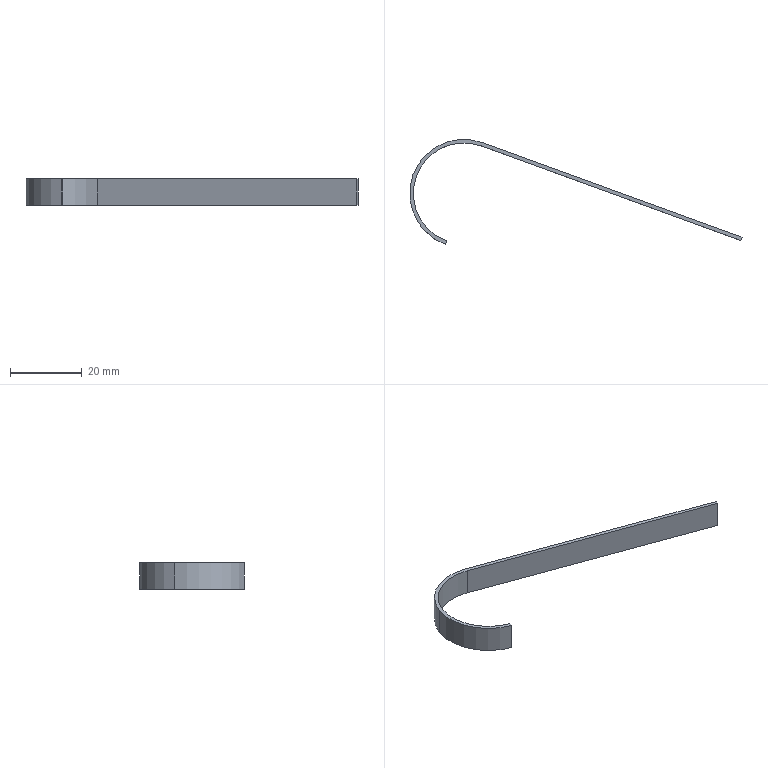Part | SolidWorks | features SplitBody 1 | 1 solid | 10 faces | box 92.373 x 29.202 x 7.5 mm | volume 918.944 mm3 | plane 6 | cylinder 4 | commonest cylinder face diameters 28.11 x2 30.11 x2
STEP:
#1=CARTESIAN_POINT('',(-138.829,345.94,-434.002));
#2=VERTEX_POINT('',#1);
#3=CARTESIAN_POINT('',(-156.843,337.54,-434.002));
#4=VERTEX_POINT('',#3);
#5=CARTESIAN_POINT('',(-143.636,332.733,-434.002));
#6=DIRECTION('',(0.,0.,1.));
#7=DIRECTION('',(0.9397,-0.342,0.));
#8=AXIS2_PLACEMENT_3D('',#5,#6,#7);
#9=CIRCLE('',#8,14.055);
#10=EDGE_CURVE('',#2,#4,#9,.T.);
#11=ORIENTED_EDGE('',*,*,#10,.T.);
#12=CARTESIAN_POINT('',(-156.843,337.54,-441.502));
#13=VERTEX_POINT('',#12);
#14=CARTESIAN_POINT('',(-156.843,337.54,-434.002));
#15=DIRECTION('',(0.,0.,-1.));
#16=VECTOR('',#15,1000.);
#17=LINE('',#14,#16);
#18=EDGE_CURVE('',#4,#13,#17,.T.);
#19=ORIENTED_EDGE('',*,*,#18,.T.);
#20=CARTESIAN_POINT('',(-138.829,345.94,-441.502));
#21=VERTEX_POINT('',#20);
#22=CARTESIAN_POINT('',(-143.636,332.733,-441.502));
#23=DIRECTION('',(0.,0.,1.));
#24=DIRECTION('',(0.9397,-0.342,0.));
#25=AXIS2_PLACEMENT_3D('',#22,#23,#24);
#26=CIRCLE('',#25,14.055);
#27=EDGE_CURVE('',#21,#13,#26,.T.);
#28=ORIENTED_EDGE('',*,*,#27,.F.);
#29=CARTESIAN_POINT('',(-138.829,345.94,-434.002));
#30=DIRECTION('',(0.,0.,-1.));
#31=VECTOR('',#30,1000.);
#32=LINE('',#29,#31);
#33=EDGE_CURVE('',#2,#21,#32,.T.);
#34=ORIENTED_EDGE('',*,*,#33,.F.);
#35=EDGE_LOOP('',(#11,#19,#28,#34));
#36=FACE_OUTER_BOUND('',#35,.T.);
#37=CARTESIAN_POINT('',(-143.636,332.733,-434.002));
#38=DIRECTION('',(0.,0.,-1.));
#39=DIRECTION('',(-0.9397,0.342,0.));
#40=AXIS2_PLACEMENT_3D('',#37,#38,#39);
#41=CYLINDRICAL_SURFACE('',#40,14.055);
#42=ADVANCED_FACE('',(#36),#41,.F.);
#43=CARTESIAN_POINT('',(-157.783,337.882,-434.002));
#44=VERTEX_POINT('',#43);
#45=CARTESIAN_POINT('',(-148.785,318.586,-434.002));
#46=VERTEX_POINT('',#45);
#47=CARTESIAN_POINT('',(-143.636,332.733,-434.002));
#48=DIRECTION('',(0.,0.,1.));
#49=DIRECTION('',(0.9397,-0.342,0.));
#50=AXIS2_PLACEMENT_3D('',#47,#48,#49);
#51=CIRCLE('',#50,15.055);
#52=EDGE_CURVE('',#44,#46,#51,.T.);
#53=ORIENTED_EDGE('',*,*,#52,.F.);
#54=CARTESIAN_POINT('',(-157.783,337.882,-441.502));
#55=VERTEX_POINT('',#54);
#56=CARTESIAN_POINT('',(-157.783,337.882,-434.002));
#57=DIRECTION('',(0.,0.,-1.));
#58=VECTOR('',#57,1000.);
#59=LINE('',#56,#58);
#60=EDGE_CURVE('',#44,#55,#59,.T.);
#61=ORIENTED_EDGE('',*,*,#60,.T.);
#62=CARTESIAN_POINT('',(-148.785,318.586,-441.502));
#63=VERTEX_POINT('',#62);
#64=CARTESIAN_POINT('',(-143.636,332.733,-441.502));
#65=DIRECTION('',(0.,0.,1.));
#66=DIRECTION('',(0.9397,-0.342,0.));
#67=AXIS2_PLACEMENT_3D('',#64,#65,#66);
#68=CIRCLE('',#67,15.055);
#69=EDGE_CURVE('',#55,#63,#68,.T.);
#70=ORIENTED_EDGE('',*,*,#69,.T.);
#71=CARTESIAN_POINT('',(-148.785,318.586,-434.002));
#72=DIRECTION('',(0.,0.,-1.));
#73=VECTOR('',#72,1000.);
#74=LINE('',#71,#73);
#75=EDGE_CURVE('',#46,#63,#74,.T.);
#76=ORIENTED_EDGE('',*,*,#75,.F.);
#77=EDGE_LOOP('',(#53,#61,#70,#76));
#78=FACE_OUTER_BOUND('',#77,.T.);
#79=CARTESIAN_POINT('',(-143.636,332.733,-434.002));
#80=DIRECTION('',(0.,0.,-1.));
#81=DIRECTION('',(-0.9397,0.342,0.));
#82=AXIS2_PLACEMENT_3D('',#79,#80,#81);
#83=CYLINDRICAL_SURFACE('',#82,15.055);
#84=ADVANCED_FACE('',(#78),#83,.T.);
#85=CARTESIAN_POINT('',(-66.66,319.673,-434.002));
#86=VERTEX_POINT('',#85);
#87=CARTESIAN_POINT('',(-138.829,345.94,-434.002));
#88=DIRECTION('',(-0.9397,0.342,0.));
#89=VECTOR('',#88,1000.);
#90=LINE('',#87,#89);
#91=EDGE_CURVE('',#86,#2,#90,.T.);
#92=ORIENTED_EDGE('',*,*,#91,.F.);
#93=CARTESIAN_POINT('',(-66.318,320.613,-434.002));
#94=VERTEX_POINT('',#93);
#95=CARTESIAN_POINT('',(-66.318,320.613,-434.002));
#96=DIRECTION('',(-0.342,-0.9397,0.));
#97=VECTOR('',#96,1000.);
#98=LINE('',#95,#97);
#99=EDGE_CURVE('',#94,#86,#98,.T.);
#100=ORIENTED_EDGE('',*,*,#99,.F.);
#101=CARTESIAN_POINT('',(-138.487,346.88,-434.002));
#102=VERTEX_POINT('',#101);
#103=CARTESIAN_POINT('',(-138.487,346.88,-434.002));
#104=DIRECTION('',(-0.9397,0.342,0.));
#105=VECTOR('',#104,1000.);
#106=LINE('',#103,#105);
#107=EDGE_CURVE('',#94,#102,#106,.T.);
#108=ORIENTED_EDGE('',*,*,#107,.T.);
#109=CARTESIAN_POINT('',(-143.636,332.733,-434.002));
#110=DIRECTION('',(0.,0.,1.));
#111=DIRECTION('',(0.9397,-0.342,0.));
#112=AXIS2_PLACEMENT_3D('',#109,#110,#111);
#113=CIRCLE('',#112,15.055);
#114=EDGE_CURVE('',#102,#44,#113,.T.);
#115=ORIENTED_EDGE('',*,*,#114,.T.);
#116=ORIENTED_EDGE('',*,*,#52,.T.);
#117=CARTESIAN_POINT('',(-148.443,319.526,-434.002));
#118=VERTEX_POINT('',#117);
#119=CARTESIAN_POINT('',(-154.581,302.663,-434.002));
#120=DIRECTION('',(0.342,0.9397,0.));
#121=VECTOR('',#120,1000.);
#122=LINE('',#119,#121);
#123=EDGE_CURVE('',#46,#118,#122,.T.);
#124=ORIENTED_EDGE('',*,*,#123,.T.);
#125=CARTESIAN_POINT('',(-143.636,332.733,-434.002));
#126=DIRECTION('',(0.,0.,1.));
#127=DIRECTION('',(0.9397,-0.342,0.));
#128=AXIS2_PLACEMENT_3D('',#125,#126,#127);
#129=CIRCLE('',#128,14.055);
#130=EDGE_CURVE('',#4,#118,#129,.T.);
#131=ORIENTED_EDGE('',*,*,#130,.F.);
#132=ORIENTED_EDGE('',*,*,#10,.F.);
#133=EDGE_LOOP('',(#92,#100,#108,#115,#116,#124,#131,#132));
#134=FACE_OUTER_BOUND('',#133,.T.);
#135=CARTESIAN_POINT('',(-143.636,332.733,-434.002));
#136=DIRECTION('',(0.,0.,1.));
#137=DIRECTION('',(0.9397,-0.342,0.));
#138=AXIS2_PLACEMENT_3D('',#135,#136,#137);
#139=PLANE('',#138);
#140=ADVANCED_FACE('',(#134),#139,.T.);
#141=CARTESIAN_POINT('',(-66.66,319.673,-441.502));
#142=VERTEX_POINT('',#141);
#143=CARTESIAN_POINT('',(-66.318,320.613,-441.502));
#144=VERTEX_POINT('',#143);
#145=CARTESIAN_POINT('',(-66.318,320.613,-441.502));
#146=DIRECTION('',(0.342,0.9397,0.));
#147=VECTOR('',#146,1000.);
#148=LINE('',#145,#147);
#149=EDGE_CURVE('',#142,#144,#148,.T.);
#150=ORIENTED_EDGE('',*,*,#149,.F.);
#151=CARTESIAN_POINT('',(-138.829,345.94,-441.502));
#152=DIRECTION('',(-0.9397,0.342,0.));
#153=VECTOR('',#152,1000.);
#154=LINE('',#151,#153);
#155=EDGE_CURVE('',#142,#21,#154,.T.);
#156=ORIENTED_EDGE('',*,*,#155,.T.);
#157=ORIENTED_EDGE('',*,*,#27,.T.);
#158=CARTESIAN_POINT('',(-148.443,319.526,-441.502));
#159=VERTEX_POINT('',#158);
#160=CARTESIAN_POINT('',(-143.636,332.733,-441.502));
#161=DIRECTION('',(0.,0.,1.));
#162=DIRECTION('',(0.9397,-0.342,0.));
#163=AXIS2_PLACEMENT_3D('',#160,#161,#162);
#164=CIRCLE('',#163,14.055);
#165=EDGE_CURVE('',#13,#159,#164,.T.);
#166=ORIENTED_EDGE('',*,*,#165,.T.);
#167=CARTESIAN_POINT('',(-154.581,302.663,-441.502));
#168=DIRECTION('',(0.342,0.9397,0.));
#169=VECTOR('',#168,1000.);
#170=LINE('',#167,#169);
#171=EDGE_CURVE('',#63,#159,#170,.T.);
#172=ORIENTED_EDGE('',*,*,#171,.F.);
#173=ORIENTED_EDGE('',*,*,#69,.F.);
#174=CARTESIAN_POINT('',(-138.487,346.88,-441.502));
#175=VERTEX_POINT('',#174);
#176=CARTESIAN_POINT('',(-143.636,332.733,-441.502));
#177=DIRECTION('',(0.,0.,1.));
#178=DIRECTION('',(0.9397,-0.342,0.));
#179=AXIS2_PLACEMENT_3D('',#176,#177,#178);
#180=CIRCLE('',#179,15.055);
#181=EDGE_CURVE('',#175,#55,#180,.T.);
#182=ORIENTED_EDGE('',*,*,#181,.F.);
#183=CARTESIAN_POINT('',(-138.487,346.88,-441.502));
#184=DIRECTION('',(-0.9397,0.342,0.));
#185=VECTOR('',#184,1000.);
#186=LINE('',#183,#185);
#187=EDGE_CURVE('',#144,#175,#186,.T.);
#188=ORIENTED_EDGE('',*,*,#187,.F.);
#189=EDGE_LOOP('',(#150,#156,#157,#166,#172,#173,#182,#188));
#190=FACE_OUTER_BOUND('',#189,.T.);
#191=CARTESIAN_POINT('',(-143.636,332.733,-441.502));
#192=DIRECTION('',(0.,0.,1.));
#193=DIRECTION('',(0.9397,-0.342,0.));
#194=AXIS2_PLACEMENT_3D('',#191,#192,#193);
#195=PLANE('',#194);
#196=ADVANCED_FACE('',(#190),#195,.F.);
#197=ORIENTED_EDGE('',*,*,#60,.F.);
#198=ORIENTED_EDGE('',*,*,#114,.F.);
#199=CARTESIAN_POINT('',(-138.487,346.88,-434.002));
#200=DIRECTION('',(0.,0.,-1.));
#201=VECTOR('',#200,1000.);
#202=LINE('',#199,#201);
#203=EDGE_CURVE('',#102,#175,#202,.T.);
#204=ORIENTED_EDGE('',*,*,#203,.T.);
#205=ORIENTED_EDGE('',*,*,#181,.T.);
#206=EDGE_LOOP('',(#197,#198,#204,#205));
#207=FACE_OUTER_BOUND('',#206,.T.);
#208=CARTESIAN_POINT('',(-143.636,332.733,-434.002));
#209=DIRECTION('',(0.,0.,-1.));
#210=DIRECTION('',(-0.9397,0.342,0.));
#211=AXIS2_PLACEMENT_3D('',#208,#209,#210);
#212=CYLINDRICAL_SURFACE('',#211,15.055);
#213=ADVANCED_FACE('',(#207),#212,.T.);
#214=ORIENTED_EDGE('',*,*,#187,.T.);
#215=ORIENTED_EDGE('',*,*,#203,.F.);
#216=ORIENTED_EDGE('',*,*,#107,.F.);
#217=CARTESIAN_POINT('',(-66.318,320.613,-434.002));
#218=DIRECTION('',(0.,0.,-1.));
#219=VECTOR('',#218,1000.);
#220=LINE('',#217,#219);
#221=EDGE_CURVE('',#94,#144,#220,.T.);
#222=ORIENTED_EDGE('',*,*,#221,.T.);
#223=EDGE_LOOP('',(#214,#215,#216,#222));
#224=FACE_OUTER_BOUND('',#223,.T.);
#225=CARTESIAN_POINT('',(-138.487,346.88,-434.002));
#226=DIRECTION('',(-0.342,-0.9397,0.));
#227=DIRECTION('',(0.9397,-0.342,0.));
#228=AXIS2_PLACEMENT_3D('',#225,#226,#227);
#229=PLANE('',#228);
#230=ADVANCED_FACE('',(#224),#229,.F.);
#231=ORIENTED_EDGE('',*,*,#18,.F.);
#232=ORIENTED_EDGE('',*,*,#130,.T.);
#233=CARTESIAN_POINT('',(-148.443,319.526,-434.002));
#234=DIRECTION('',(0.,0.,-1.));
#235=VECTOR('',#234,1000.);
#236=LINE('',#233,#235);
#237=EDGE_CURVE('',#118,#159,#236,.T.);
#238=ORIENTED_EDGE('',*,*,#237,.T.);
#239=ORIENTED_EDGE('',*,*,#165,.F.);
#240=EDGE_LOOP('',(#231,#232,#238,#239));
#241=FACE_OUTER_BOUND('',#240,.T.);
#242=CARTESIAN_POINT('',(-143.636,332.733,-434.002));
#243=DIRECTION('',(0.,0.,-1.));
#244=DIRECTION('',(-0.9397,0.342,0.));
#245=AXIS2_PLACEMENT_3D('',#242,#243,#244);
#246=CYLINDRICAL_SURFACE('',#245,14.055);
#247=ADVANCED_FACE('',(#241),#246,.F.);
#248=ORIENTED_EDGE('',*,*,#155,.F.);
#249=CARTESIAN_POINT('',(-66.66,319.673,-434.002));
#250=DIRECTION('',(0.,0.,-1.));
#251=VECTOR('',#250,1000.);
#252=LINE('',#249,#251);
#253=EDGE_CURVE('',#86,#142,#252,.T.);
#254=ORIENTED_EDGE('',*,*,#253,.F.);
#255=ORIENTED_EDGE('',*,*,#91,.T.);
#256=ORIENTED_EDGE('',*,*,#33,.T.);
#257=EDGE_LOOP('',(#248,#254,#255,#256));
#258=FACE_OUTER_BOUND('',#257,.T.);
#259=CARTESIAN_POINT('',(-138.829,345.94,-434.002));
#260=DIRECTION('',(-0.342,-0.9397,0.));
#261=DIRECTION('',(0.9397,-0.342,0.));
#262=AXIS2_PLACEMENT_3D('',#259,#260,#261);
#263=PLANE('',#262);
#264=ADVANCED_FACE('',(#258),#263,.T.);
#265=ORIENTED_EDGE('',*,*,#171,.T.);
#266=ORIENTED_EDGE('',*,*,#237,.F.);
#267=ORIENTED_EDGE('',*,*,#123,.F.);
#268=ORIENTED_EDGE('',*,*,#75,.T.);
#269=EDGE_LOOP('',(#265,#266,#267,#268));
#270=FACE_OUTER_BOUND('',#269,.T.);
#271=CARTESIAN_POINT('',(-154.581,302.663,-441.502));
#272=DIRECTION('',(-0.9397,0.342,0.));
#273=DIRECTION('',(0.,0.,1.));
#274=AXIS2_PLACEMENT_3D('',#271,#272,#273);
#275=PLANE('',#274);
#276=ADVANCED_FACE('',(#270),#275,.F.);
#277=ORIENTED_EDGE('',*,*,#149,.T.);
#278=ORIENTED_EDGE('',*,*,#221,.F.);
#279=ORIENTED_EDGE('',*,*,#99,.T.);
#280=ORIENTED_EDGE('',*,*,#253,.T.);
#281=EDGE_LOOP('',(#277,#278,#279,#280));
#282=FACE_OUTER_BOUND('',#281,.T.);
#283=CARTESIAN_POINT('',(-71.468,306.466,-437.752));
#284=DIRECTION('',(0.9397,-0.342,0.));
#285=DIRECTION('',(0.,0.,-1.));
#286=AXIS2_PLACEMENT_3D('',#283,#284,#285);
#287=PLANE('',#286);
#288=ADVANCED_FACE('',(#282),#287,.T.);
#289=CLOSED_SHELL('',(#42,#84,#140,#196,#213,#230,#247,#264,#276,#288));
#290=MANIFOLD_SOLID_BREP('',#289);
#291=CARTESIAN_POINT('',(0.,0.,0.));
#292=DIRECTION('',(0.,0.,1.));
#293=DIRECTION('',(1.,0.,0.));
#294=AXIS2_PLACEMENT_3D('',#291,#292,#293);
#295=(LENGTH_UNIT()NAMED_UNIT(*)SI_UNIT(.MILLI.,.METRE.));
#296=UNCERTAINTY_MEASURE_WITH_UNIT(LENGTH_MEASURE(0.00001),#295,'','');
#297=(NAMED_UNIT(*)PLANE_ANGLE_UNIT()SI_UNIT($,.RADIAN.));
#298=(NAMED_UNIT(*)SI_UNIT($,.STERADIAN.)SOLID_ANGLE_UNIT());
#299=(GEOMETRIC_REPRESENTATION_CONTEXT(3)GLOBAL_UNCERTAINTY_ASSIGNED_CONTEXT((#296))GLOBAL_UNIT_ASSIGNED_CONTEXT((#295,#297,#298))REPRESENTATION_CONTEXT('',''));
#300=ADVANCED_BREP_SHAPE_REPRESENTATION('',(#290,#294),#299);